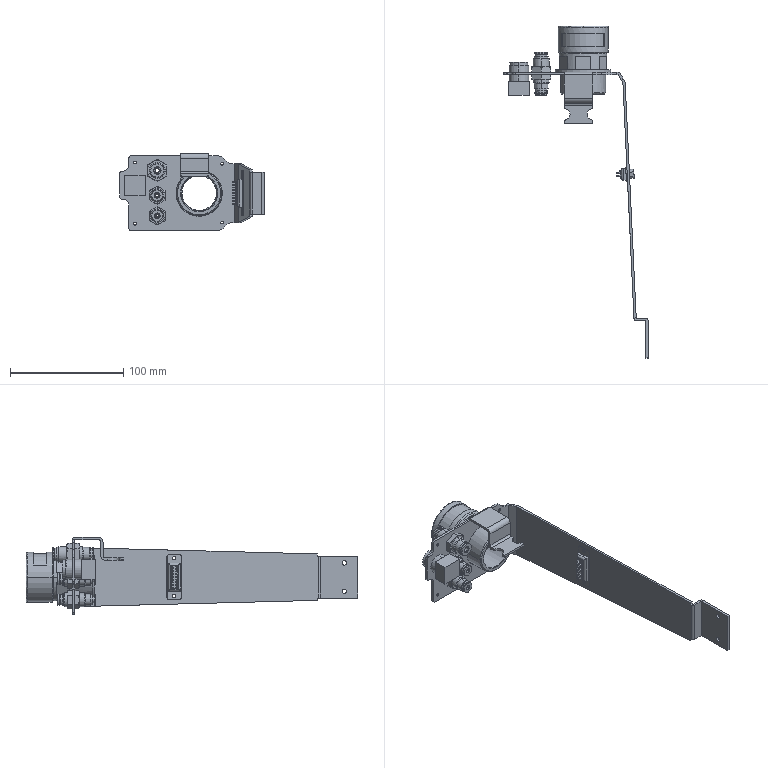Part | STEP file | 11-Cover41111 | 4 solids | 659 faces | box 127.366 x 293 x 68 mm | volume 86944 mm3 | plane 350 | cylinder 216 | cone 91 | torus 2 | commonest cylinder face diameters 1 x35 4 x24 12 x12 2 x10 2.459 x8 5 x8